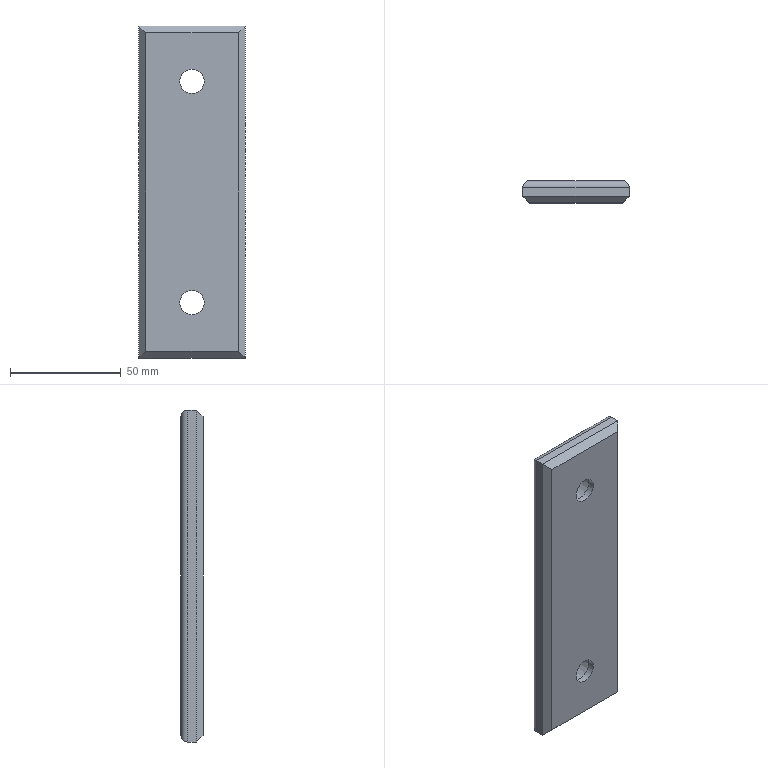Part | NX | features solid 2 | 1 solid | 20 faces | box 48 x 10 x 150 mm | volume 65562 mm3 | plane 12 | cylinder 8 | commonest cylinder face diameters 6 x4 11 x2 17.5 x2
STEP:
#1=CARTESIAN_POINT('',(95.,448.,45.));
#2=VERTEX_POINT('',#1);
#3=CARTESIAN_POINT('',(95.,452.,45.));
#4=VERTEX_POINT('',#3);
#5=CARTESIAN_POINT('',(95.,445.,45.));
#6=DIRECTION('',(0.,1.,0.));
#7=VECTOR('',#6,1000.);
#8=LINE('',#5,#7);
#9=EDGE_CURVE('',#2,#4,#8,.T.);
#10=ORIENTED_EDGE('',*,*,#9,.T.);
#11=CARTESIAN_POINT('',(143.,452.,45.));
#12=VERTEX_POINT('',#11);
#13=CARTESIAN_POINT('',(143.,452.,45.));
#14=DIRECTION('',(-1.,0.,0.));
#15=VECTOR('',#14,1000.);
#16=LINE('',#13,#15);
#17=EDGE_CURVE('',#12,#4,#16,.T.);
#18=ORIENTED_EDGE('',*,*,#17,.F.);
#19=CARTESIAN_POINT('',(143.,448.,45.));
#20=VERTEX_POINT('',#19);
#21=CARTESIAN_POINT('',(143.,445.,45.));
#22=DIRECTION('',(0.,1.,0.));
#23=VECTOR('',#22,1000.);
#24=LINE('',#21,#23);
#25=EDGE_CURVE('',#20,#12,#24,.T.);
#26=ORIENTED_EDGE('',*,*,#25,.F.);
#27=CARTESIAN_POINT('',(143.,448.,45.));
#28=DIRECTION('',(1.,0.,0.));
#29=VECTOR('',#28,1000.);
#30=LINE('',#27,#29);
#31=EDGE_CURVE('',#2,#20,#30,.T.);
#32=ORIENTED_EDGE('',*,*,#31,.F.);
#33=EDGE_LOOP('',(#10,#18,#26,#32));
#34=FACE_BOUND('',#33,.T.);
#35=CARTESIAN_POINT('',(143.,445.,45.));
#36=DIRECTION('',(0.,0.,1.));
#37=DIRECTION('',(0.,1.,0.));
#38=AXIS2_PLACEMENT_3D('',#35,#36,#37);
#39=PLANE('',#38);
#40=ADVANCED_FACE('',(#34),#39,.F.);
#41=CARTESIAN_POINT('',(95.,448.,195.));
#42=VERTEX_POINT('',#41);
#43=CARTESIAN_POINT('',(95.,452.,195.));
#44=VERTEX_POINT('',#43);
#45=CARTESIAN_POINT('',(95.,445.,195.));
#46=DIRECTION('',(0.,1.,0.));
#47=VECTOR('',#46,1000.);
#48=LINE('',#45,#47);
#49=EDGE_CURVE('',#42,#44,#48,.T.);
#50=ORIENTED_EDGE('',*,*,#49,.T.);
#51=CARTESIAN_POINT('',(95.,452.,45.));
#52=DIRECTION('',(0.,0.,1.));
#53=VECTOR('',#52,1000.);
#54=LINE('',#51,#53);
#55=EDGE_CURVE('',#4,#44,#54,.T.);
#56=ORIENTED_EDGE('',*,*,#55,.F.);
#57=ORIENTED_EDGE('',*,*,#9,.F.);
#58=CARTESIAN_POINT('',(95.,448.,45.));
#59=DIRECTION('',(0.,0.,-1.));
#60=VECTOR('',#59,1000.);
#61=LINE('',#58,#60);
#62=EDGE_CURVE('',#42,#2,#61,.T.);
#63=ORIENTED_EDGE('',*,*,#62,.F.);
#64=EDGE_LOOP('',(#50,#56,#57,#63));
#65=FACE_BOUND('',#64,.T.);
#66=CARTESIAN_POINT('',(95.,445.,45.));
#67=DIRECTION('',(1.,0.,0.));
#68=DIRECTION('',(0.,-1.,0.));
#69=AXIS2_PLACEMENT_3D('',#66,#67,#68);
#70=PLANE('',#69);
#71=ADVANCED_FACE('',(#65),#70,.F.);
#72=CARTESIAN_POINT('',(143.,448.,195.));
#73=VERTEX_POINT('',#72);
#74=CARTESIAN_POINT('',(143.,452.,195.));
#75=VERTEX_POINT('',#74);
#76=CARTESIAN_POINT('',(143.,445.,195.));
#77=DIRECTION('',(0.,1.,0.));
#78=VECTOR('',#77,1000.);
#79=LINE('',#76,#78);
#80=EDGE_CURVE('',#73,#75,#79,.T.);
#81=ORIENTED_EDGE('',*,*,#80,.T.);
#82=CARTESIAN_POINT('',(95.,452.,195.));
#83=DIRECTION('',(1.,0.,0.));
#84=VECTOR('',#83,1000.);
#85=LINE('',#82,#84);
#86=EDGE_CURVE('',#44,#75,#85,.T.);
#87=ORIENTED_EDGE('',*,*,#86,.F.);
#88=ORIENTED_EDGE('',*,*,#49,.F.);
#89=CARTESIAN_POINT('',(95.,448.,195.));
#90=DIRECTION('',(-1.,0.,0.));
#91=VECTOR('',#90,1000.);
#92=LINE('',#89,#91);
#93=EDGE_CURVE('',#73,#42,#92,.T.);
#94=ORIENTED_EDGE('',*,*,#93,.F.);
#95=EDGE_LOOP('',(#81,#87,#88,#94));
#96=FACE_BOUND('',#95,.T.);
#97=CARTESIAN_POINT('',(95.,445.,195.));
#98=DIRECTION('',(0.,0.,-1.));
#99=DIRECTION('',(-1.,0.,0.));
#100=AXIS2_PLACEMENT_3D('',#97,#98,#99);
#101=PLANE('',#100);
#102=ADVANCED_FACE('',(#96),#101,.F.);
#103=ORIENTED_EDGE('',*,*,#25,.T.);
#104=CARTESIAN_POINT('',(143.,452.,145.));
#105=DIRECTION('',(0.,0.,-1.));
#106=VECTOR('',#105,1000.);
#107=LINE('',#104,#106);
#108=EDGE_CURVE('',#75,#12,#107,.T.);
#109=ORIENTED_EDGE('',*,*,#108,.F.);
#110=ORIENTED_EDGE('',*,*,#80,.F.);
#111=CARTESIAN_POINT('',(143.,448.,145.));
#112=DIRECTION('',(0.,0.,1.));
#113=VECTOR('',#112,1000.);
#114=LINE('',#111,#113);
#115=EDGE_CURVE('',#20,#73,#114,.T.);
#116=ORIENTED_EDGE('',*,*,#115,.F.);
#117=EDGE_LOOP('',(#103,#109,#110,#116));
#118=FACE_BOUND('',#117,.T.);
#119=CARTESIAN_POINT('',(143.,445.,145.));
#120=DIRECTION('',(-1.,0.,0.));
#121=DIRECTION('',(0.,0.,1.));
#122=AXIS2_PLACEMENT_3D('',#119,#120,#121);
#123=PLANE('',#122);
#124=ADVANCED_FACE('',(#118),#123,.F.);
#125=CARTESIAN_POINT('',(98.,445.,48.));
#126=VERTEX_POINT('',#125);
#127=CARTESIAN_POINT('',(98.,445.,192.));
#128=VERTEX_POINT('',#127);
#129=CARTESIAN_POINT('',(98.,445.,145.));
#130=DIRECTION('',(0.,0.,1.));
#131=VECTOR('',#130,1000.);
#132=LINE('',#129,#131);
#133=EDGE_CURVE('',#126,#128,#132,.T.);
#134=ORIENTED_EDGE('',*,*,#133,.F.);
#135=CARTESIAN_POINT('',(140.,445.,48.));
#136=VERTEX_POINT('',#135);
#137=CARTESIAN_POINT('',(95.,445.,48.));
#138=DIRECTION('',(-1.,0.,0.));
#139=VECTOR('',#138,1000.);
#140=LINE('',#137,#139);
#141=EDGE_CURVE('',#136,#126,#140,.T.);
#142=ORIENTED_EDGE('',*,*,#141,.F.);
#143=CARTESIAN_POINT('',(140.,445.,192.));
#144=VERTEX_POINT('',#143);
#145=CARTESIAN_POINT('',(140.,445.,45.));
#146=DIRECTION('',(0.,0.,-1.));
#147=VECTOR('',#146,1000.);
#148=LINE('',#145,#147);
#149=EDGE_CURVE('',#144,#136,#148,.T.);
#150=ORIENTED_EDGE('',*,*,#149,.F.);
#151=CARTESIAN_POINT('',(143.,445.,192.));
#152=DIRECTION('',(1.,0.,0.));
#153=VECTOR('',#152,1000.);
#154=LINE('',#151,#153);
#155=EDGE_CURVE('',#128,#144,#154,.T.);
#156=ORIENTED_EDGE('',*,*,#155,.F.);
#157=EDGE_LOOP('',(#134,#142,#150,#156));
#158=FACE_BOUND('',#157,.T.);
#159=CARTESIAN_POINT('',(119.,445.,175.5));
#160=VERTEX_POINT('',#159);
#161=CARTESIAN_POINT('',(119.,445.,170.));
#162=DIRECTION('',(0.,1.,0.));
#163=DIRECTION('',(0.,0.,1.));
#164=AXIS2_PLACEMENT_3D('',#161,#162,#163);
#165=CIRCLE('',#164,5.5);
#166=EDGE_CURVE('',#160,#160,#165,.T.);
#167=ORIENTED_EDGE('',*,*,#166,.T.);
#168=EDGE_LOOP('',(#167));
#169=FACE_BOUND('',#168,.T.);
#170=CARTESIAN_POINT('',(119.,445.,75.5));
#171=VERTEX_POINT('',#170);
#172=CARTESIAN_POINT('',(119.,445.,70.));
#173=DIRECTION('',(0.,1.,0.));
#174=DIRECTION('',(0.,0.,1.));
#175=AXIS2_PLACEMENT_3D('',#172,#173,#174);
#176=CIRCLE('',#175,5.5);
#177=EDGE_CURVE('',#171,#171,#176,.T.);
#178=ORIENTED_EDGE('',*,*,#177,.T.);
#179=EDGE_LOOP('',(#178));
#180=FACE_BOUND('',#179,.T.);
#181=CARTESIAN_POINT('',(95.,445.,45.));
#182=DIRECTION('',(0.,-1.,0.));
#183=DIRECTION('',(0.,0.,1.));
#184=AXIS2_PLACEMENT_3D('',#181,#182,#183);
#185=PLANE('',#184);
#186=ADVANCED_FACE('',(#158,#169,#180),#185,.T.);
#187=CARTESIAN_POINT('',(98.,455.,48.));
#188=VERTEX_POINT('',#187);
#189=CARTESIAN_POINT('',(140.,455.,48.));
#190=VERTEX_POINT('',#189);
#191=CARTESIAN_POINT('',(95.,455.,48.));
#192=DIRECTION('',(-1.,0.,0.));
#193=VECTOR('',#192,1000.);
#194=LINE('',#191,#193);
#195=EDGE_CURVE('',#188,#190,#194,.F.);
#196=ORIENTED_EDGE('',*,*,#195,.F.);
#197=CARTESIAN_POINT('',(98.,455.,192.));
#198=VERTEX_POINT('',#197);
#199=CARTESIAN_POINT('',(98.,455.,45.));
#200=DIRECTION('',(0.,0.,1.));
#201=VECTOR('',#200,1000.);
#202=LINE('',#199,#201);
#203=EDGE_CURVE('',#198,#188,#202,.F.);
#204=ORIENTED_EDGE('',*,*,#203,.F.);
#205=CARTESIAN_POINT('',(140.,455.,192.));
#206=VERTEX_POINT('',#205);
#207=CARTESIAN_POINT('',(95.,455.,192.));
#208=DIRECTION('',(1.,0.,0.));
#209=VECTOR('',#208,1000.);
#210=LINE('',#207,#209);
#211=EDGE_CURVE('',#206,#198,#210,.F.);
#212=ORIENTED_EDGE('',*,*,#211,.F.);
#213=CARTESIAN_POINT('',(140.,455.,45.));
#214=DIRECTION('',(0.,0.,-1.));
#215=VECTOR('',#214,1000.);
#216=LINE('',#213,#215);
#217=EDGE_CURVE('',#190,#206,#216,.F.);
#218=ORIENTED_EDGE('',*,*,#217,.F.);
#219=EDGE_LOOP('',(#196,#204,#212,#218));
#220=FACE_BOUND('',#219,.T.);
#221=CARTESIAN_POINT('',(119.,455.,178.75));
#222=VERTEX_POINT('',#221);
#223=CARTESIAN_POINT('',(119.,455.,170.));
#224=DIRECTION('',(0.,1.,0.));
#225=DIRECTION('',(0.,0.,1.));
#226=AXIS2_PLACEMENT_3D('',#223,#224,#225);
#227=CIRCLE('',#226,8.75);
#228=EDGE_CURVE('',#222,#222,#227,.T.);
#229=ORIENTED_EDGE('',*,*,#228,.F.);
#230=EDGE_LOOP('',(#229));
#231=FACE_BOUND('',#230,.T.);
#232=CARTESIAN_POINT('',(119.,455.,78.75));
#233=VERTEX_POINT('',#232);
#234=CARTESIAN_POINT('',(119.,455.,70.));
#235=DIRECTION('',(0.,1.,0.));
#236=DIRECTION('',(0.,0.,1.));
#237=AXIS2_PLACEMENT_3D('',#234,#235,#236);
#238=CIRCLE('',#237,8.75);
#239=EDGE_CURVE('',#233,#233,#238,.T.);
#240=ORIENTED_EDGE('',*,*,#239,.F.);
#241=EDGE_LOOP('',(#240));
#242=FACE_BOUND('',#241,.T.);
#243=CARTESIAN_POINT('',(95.,455.,45.));
#244=DIRECTION('',(0.,-1.,0.));
#245=DIRECTION('',(0.,0.,1.));
#246=AXIS2_PLACEMENT_3D('',#243,#244,#245);
#247=PLANE('',#246);
#248=ADVANCED_FACE('',(#220,#231,#242),#247,.F.);
#249=ORIENTED_EDGE('',*,*,#177,.F.);
#250=EDGE_LOOP('',(#249));
#251=FACE_BOUND('',#250,.T.);
#252=CARTESIAN_POINT('',(119.,448.,64.5));
#253=VERTEX_POINT('',#252);
#254=CARTESIAN_POINT('',(119.,448.,70.));
#255=DIRECTION('',(0.,1.,0.));
#256=DIRECTION('',(0.,0.,-1.));
#257=AXIS2_PLACEMENT_3D('',#254,#255,#256);
#258=CIRCLE('',#257,5.5);
#259=EDGE_CURVE('',#253,#253,#258,.T.);
#260=ORIENTED_EDGE('',*,*,#259,.T.);
#261=EDGE_LOOP('',(#260));
#262=FACE_BOUND('',#261,.T.);
#263=CARTESIAN_POINT('',(119.,415.,70.));
#264=DIRECTION('',(0.,-1.,0.));
#265=DIRECTION('',(0.,0.,1.));
#266=AXIS2_PLACEMENT_3D('',#263,#264,#265);
#267=CYLINDRICAL_SURFACE('',#266,5.5);
#268=ADVANCED_FACE('',(#251,#262),#267,.F.);
#269=ORIENTED_EDGE('',*,*,#259,.F.);
#270=EDGE_LOOP('',(#269));
#271=FACE_BOUND('',#270,.T.);
#272=CARTESIAN_POINT('',(119.,448.,61.25));
#273=VERTEX_POINT('',#272);
#274=CARTESIAN_POINT('',(119.,448.,70.));
#275=DIRECTION('',(0.,1.,0.));
#276=DIRECTION('',(0.,0.,-1.));
#277=AXIS2_PLACEMENT_3D('',#274,#275,#276);
#278=CIRCLE('',#277,8.75);
#279=EDGE_CURVE('',#273,#273,#278,.T.);
#280=ORIENTED_EDGE('',*,*,#279,.T.);
#281=EDGE_LOOP('',(#280));
#282=FACE_BOUND('',#281,.T.);
#283=CARTESIAN_POINT('',(119.,448.,70.));
#284=DIRECTION('',(0.,-1.,0.));
#285=DIRECTION('',(0.,0.,1.));
#286=AXIS2_PLACEMENT_3D('',#283,#284,#285);
#287=PLANE('',#286);
#288=ADVANCED_FACE('',(#271,#282),#287,.F.);
#289=ORIENTED_EDGE('',*,*,#279,.F.);
#290=EDGE_LOOP('',(#289));
#291=FACE_BOUND('',#290,.T.);
#292=ORIENTED_EDGE('',*,*,#239,.T.);
#293=EDGE_LOOP('',(#292));
#294=FACE_BOUND('',#293,.T.);
#295=CARTESIAN_POINT('',(119.,465.,70.));
#296=DIRECTION('',(0.,-1.,0.));
#297=DIRECTION('',(0.,0.,1.));
#298=AXIS2_PLACEMENT_3D('',#295,#296,#297);
#299=CYLINDRICAL_SURFACE('',#298,8.75);
#300=ADVANCED_FACE('',(#291,#294),#299,.F.);
#301=ORIENTED_EDGE('',*,*,#166,.F.);
#302=EDGE_LOOP('',(#301));
#303=FACE_BOUND('',#302,.T.);
#304=CARTESIAN_POINT('',(119.,448.,164.5));
#305=VERTEX_POINT('',#304);
#306=CARTESIAN_POINT('',(119.,448.,170.));
#307=DIRECTION('',(0.,1.,0.));
#308=DIRECTION('',(0.,0.,-1.));
#309=AXIS2_PLACEMENT_3D('',#306,#307,#308);
#310=CIRCLE('',#309,5.5);
#311=EDGE_CURVE('',#305,#305,#310,.T.);
#312=ORIENTED_EDGE('',*,*,#311,.T.);
#313=EDGE_LOOP('',(#312));
#314=FACE_BOUND('',#313,.T.);
#315=CARTESIAN_POINT('',(119.,415.,170.));
#316=DIRECTION('',(0.,-1.,0.));
#317=DIRECTION('',(0.,0.,1.));
#318=AXIS2_PLACEMENT_3D('',#315,#316,#317);
#319=CYLINDRICAL_SURFACE('',#318,5.5);
#320=ADVANCED_FACE('',(#303,#314),#319,.F.);
#321=ORIENTED_EDGE('',*,*,#311,.F.);
#322=EDGE_LOOP('',(#321));
#323=FACE_BOUND('',#322,.T.);
#324=CARTESIAN_POINT('',(119.,448.,161.25));
#325=VERTEX_POINT('',#324);
#326=CARTESIAN_POINT('',(119.,448.,170.));
#327=DIRECTION('',(0.,1.,0.));
#328=DIRECTION('',(0.,0.,-1.));
#329=AXIS2_PLACEMENT_3D('',#326,#327,#328);
#330=CIRCLE('',#329,8.75);
#331=EDGE_CURVE('',#325,#325,#330,.T.);
#332=ORIENTED_EDGE('',*,*,#331,.T.);
#333=EDGE_LOOP('',(#332));
#334=FACE_BOUND('',#333,.T.);
#335=CARTESIAN_POINT('',(119.,448.,120.));
#336=DIRECTION('',(0.,-1.,0.));
#337=DIRECTION('',(0.,0.,1.));
#338=AXIS2_PLACEMENT_3D('',#335,#336,#337);
#339=PLANE('',#338);
#340=ADVANCED_FACE('',(#323,#334),#339,.F.);
#341=ORIENTED_EDGE('',*,*,#331,.F.);
#342=EDGE_LOOP('',(#341));
#343=FACE_BOUND('',#342,.T.);
#344=ORIENTED_EDGE('',*,*,#228,.T.);
#345=EDGE_LOOP('',(#344));
#346=FACE_BOUND('',#345,.T.);
#347=CARTESIAN_POINT('',(119.,465.,170.));
#348=DIRECTION('',(0.,-1.,0.));
#349=DIRECTION('',(0.,0.,1.));
#350=AXIS2_PLACEMENT_3D('',#347,#348,#349);
#351=CYLINDRICAL_SURFACE('',#350,8.75);
#352=ADVANCED_FACE('',(#343,#346),#351,.F.);
#353=CARTESIAN_POINT('',(98.,452.,48.));
#354=DIRECTION('',(0.7071,0.,-0.7071));
#355=DIRECTION('',(-0.7071,0.,-0.7071));
#356=AXIS2_PLACEMENT_3D('',#353,#354,#355);
#357=ELLIPSE('',#356,4.243,3.);
#358=EDGE_CURVE('',#188,#4,#357,.F.);
#359=ORIENTED_EDGE('',*,*,#358,.T.);
#360=ORIENTED_EDGE('',*,*,#55,.T.);
#361=CARTESIAN_POINT('',(98.,452.,192.));
#362=DIRECTION('',(-0.7071,0.,-0.7071));
#363=DIRECTION('',(-0.7071,0.,0.7071));
#364=AXIS2_PLACEMENT_3D('',#361,#362,#363);
#365=ELLIPSE('',#364,4.243,3.);
#366=EDGE_CURVE('',#44,#198,#365,.T.);
#367=ORIENTED_EDGE('',*,*,#366,.T.);
#368=ORIENTED_EDGE('',*,*,#203,.T.);
#369=EDGE_LOOP('',(#359,#360,#367,#368));
#370=FACE_BOUND('',#369,.T.);
#371=CARTESIAN_POINT('',(98.,452.,45.));
#372=DIRECTION('',(0.,0.,1.));
#373=DIRECTION('',(0.,1.,0.));
#374=AXIS2_PLACEMENT_3D('',#371,#372,#373);
#375=CYLINDRICAL_SURFACE('',#374,3.);
#376=ADVANCED_FACE('',(#370),#375,.T.);
#377=ORIENTED_EDGE('',*,*,#366,.F.);
#378=ORIENTED_EDGE('',*,*,#86,.T.);
#379=CARTESIAN_POINT('',(140.,452.,192.));
#380=DIRECTION('',(-0.7071,0.,0.7071));
#381=DIRECTION('',(0.7071,0.,0.7071));
#382=AXIS2_PLACEMENT_3D('',#379,#380,#381);
#383=ELLIPSE('',#382,4.243,3.);
#384=EDGE_CURVE('',#75,#206,#383,.T.);
#385=ORIENTED_EDGE('',*,*,#384,.T.);
#386=ORIENTED_EDGE('',*,*,#211,.T.);
#387=EDGE_LOOP('',(#377,#378,#385,#386));
#388=FACE_BOUND('',#387,.T.);
#389=CARTESIAN_POINT('',(95.,452.,192.));
#390=DIRECTION('',(1.,0.,0.));
#391=DIRECTION('',(0.,0.,-1.));
#392=AXIS2_PLACEMENT_3D('',#389,#390,#391);
#393=CYLINDRICAL_SURFACE('',#392,3.);
#394=ADVANCED_FACE('',(#388),#393,.T.);
#395=ORIENTED_EDGE('',*,*,#358,.F.);
#396=ORIENTED_EDGE('',*,*,#195,.T.);
#397=CARTESIAN_POINT('',(140.,452.,48.));
#398=DIRECTION('',(0.7071,0.,0.7071));
#399=DIRECTION('',(-0.7071,0.,0.7071));
#400=AXIS2_PLACEMENT_3D('',#397,#398,#399);
#401=ELLIPSE('',#400,4.243,3.);
#402=EDGE_CURVE('',#190,#12,#401,.F.);
#403=ORIENTED_EDGE('',*,*,#402,.T.);
#404=ORIENTED_EDGE('',*,*,#17,.T.);
#405=EDGE_LOOP('',(#395,#396,#403,#404));
#406=FACE_BOUND('',#405,.T.);
#407=CARTESIAN_POINT('',(143.,452.,48.));
#408=DIRECTION('',(-1.,0.,0.));
#409=DIRECTION('',(0.,1.,0.));
#410=AXIS2_PLACEMENT_3D('',#407,#408,#409);
#411=CYLINDRICAL_SURFACE('',#410,3.);
#412=ADVANCED_FACE('',(#406),#411,.T.);
#413=ORIENTED_EDGE('',*,*,#384,.F.);
#414=ORIENTED_EDGE('',*,*,#108,.T.);
#415=ORIENTED_EDGE('',*,*,#402,.F.);
#416=ORIENTED_EDGE('',*,*,#217,.T.);
#417=EDGE_LOOP('',(#413,#414,#415,#416));
#418=FACE_BOUND('',#417,.T.);
#419=CARTESIAN_POINT('',(140.,452.,145.));
#420=DIRECTION('',(0.,0.,-1.));
#421=DIRECTION('',(-1.,0.,0.));
#422=AXIS2_PLACEMENT_3D('',#419,#420,#421);
#423=CYLINDRICAL_SURFACE('',#422,3.);
#424=ADVANCED_FACE('',(#418),#423,.T.);
#425=CARTESIAN_POINT('',(141.,446.,47.));
#426=DIRECTION('',(-0.5774,-0.5774,0.5774));
#427=VECTOR('',#426,1000.);
#428=LINE('',#425,#427);
#429=EDGE_CURVE('',#20,#136,#428,.T.);
#430=ORIENTED_EDGE('',*,*,#429,.T.);
#431=ORIENTED_EDGE('',*,*,#141,.T.);
#432=CARTESIAN_POINT('',(97.,446.,47.));
#433=DIRECTION('',(0.5774,-0.5774,0.5774));
#434=VECTOR('',#433,1000.);
#435=LINE('',#432,#434);
#436=EDGE_CURVE('',#126,#2,#435,.F.);
#437=ORIENTED_EDGE('',*,*,#436,.T.);
#438=ORIENTED_EDGE('',*,*,#31,.T.);
#439=EDGE_LOOP('',(#430,#431,#437,#438));
#440=FACE_BOUND('',#439,.T.);
#441=CARTESIAN_POINT('',(95.,445.,48.));
#442=DIRECTION('',(0.,-0.7071,-0.7071));
#443=DIRECTION('',(0.,-0.7071,0.7071));
#444=AXIS2_PLACEMENT_3D('',#441,#442,#443);
#445=PLANE('',#444);
#446=ADVANCED_FACE('',(#440),#445,.T.);
#447=ORIENTED_EDGE('',*,*,#436,.F.);
#448=ORIENTED_EDGE('',*,*,#133,.T.);
#449=CARTESIAN_POINT('',(130.333,412.667,159.667));
#450=DIRECTION('',(0.5774,-0.5774,-0.5774));
#451=VECTOR('',#450,1000.);
#452=LINE('',#449,#451);
#453=EDGE_CURVE('',#128,#42,#452,.F.);
#454=ORIENTED_EDGE('',*,*,#453,.T.);
#455=ORIENTED_EDGE('',*,*,#62,.T.);
#456=EDGE_LOOP('',(#447,#448,#454,#455));
#457=FACE_BOUND('',#456,.T.);
#458=CARTESIAN_POINT('',(98.,445.,45.));
#459=DIRECTION('',(-0.7071,-0.7071,0.));
#460=DIRECTION('',(-0.7071,0.7071,0.));
#461=AXIS2_PLACEMENT_3D('',#458,#459,#460);
#462=PLANE('',#461);
#463=ADVANCED_FACE('',(#457),#462,.T.);
#464=ORIENTED_EDGE('',*,*,#429,.F.);
#465=ORIENTED_EDGE('',*,*,#115,.T.);
#466=CARTESIAN_POINT('',(107.667,412.667,159.667));
#467=DIRECTION('',(0.5774,0.5774,0.5774));
#468=VECTOR('',#467,1000.);
#469=LINE('',#466,#468);
#470=EDGE_CURVE('',#73,#144,#469,.F.);
#471=ORIENTED_EDGE('',*,*,#470,.T.);
#472=ORIENTED_EDGE('',*,*,#149,.T.);
#473=EDGE_LOOP('',(#464,#465,#471,#472));
#474=FACE_BOUND('',#473,.T.);
#475=CARTESIAN_POINT('',(140.,445.,45.));
#476=DIRECTION('',(0.7071,-0.7071,0.));
#477=DIRECTION('',(-0.7071,-0.7071,0.));
#478=AXIS2_PLACEMENT_3D('',#475,#476,#477);
#479=PLANE('',#478);
#480=ADVANCED_FACE('',(#474),#479,.T.);
#481=ORIENTED_EDGE('',*,*,#453,.F.);
#482=ORIENTED_EDGE('',*,*,#155,.T.);
#483=ORIENTED_EDGE('',*,*,#470,.F.);
#484=ORIENTED_EDGE('',*,*,#93,.T.);
#485=EDGE_LOOP('',(#481,#482,#483,#484));
#486=FACE_BOUND('',#485,.T.);
#487=CARTESIAN_POINT('',(95.,445.,192.));
#488=DIRECTION('',(0.,-0.7071,0.7071));
#489=DIRECTION('',(0.,0.7071,0.7071));
#490=AXIS2_PLACEMENT_3D('',#487,#488,#489);
#491=PLANE('',#490);
#492=ADVANCED_FACE('',(#486),#491,.T.);
#493=CLOSED_SHELL('',(#40,#71,#102,#124,#186,#248,#268,#288,#300,#320,#340,#352,#376,#394,#412,#424,#446,#463,#480,#492));
#494=MANIFOLD_SOLID_BREP('',#493);
#495=(LENGTH_UNIT()NAMED_UNIT(*)SI_UNIT(.MILLI.,.METRE.));
#496=UNCERTAINTY_MEASURE_WITH_UNIT(LENGTH_MEASURE(0.00001),#495,'','');
#497=(NAMED_UNIT(*)PLANE_ANGLE_UNIT()SI_UNIT($,.RADIAN.));
#498=(NAMED_UNIT(*)SI_UNIT($,.STERADIAN.)SOLID_ANGLE_UNIT());
#499=(GEOMETRIC_REPRESENTATION_CONTEXT(3)GLOBAL_UNCERTAINTY_ASSIGNED_CONTEXT((#496))GLOBAL_UNIT_ASSIGNED_CONTEXT((#495,#497,#498))REPRESENTATION_CONTEXT('',''));
#500=ADVANCED_BREP_SHAPE_REPRESENTATION('',(#494),#499);